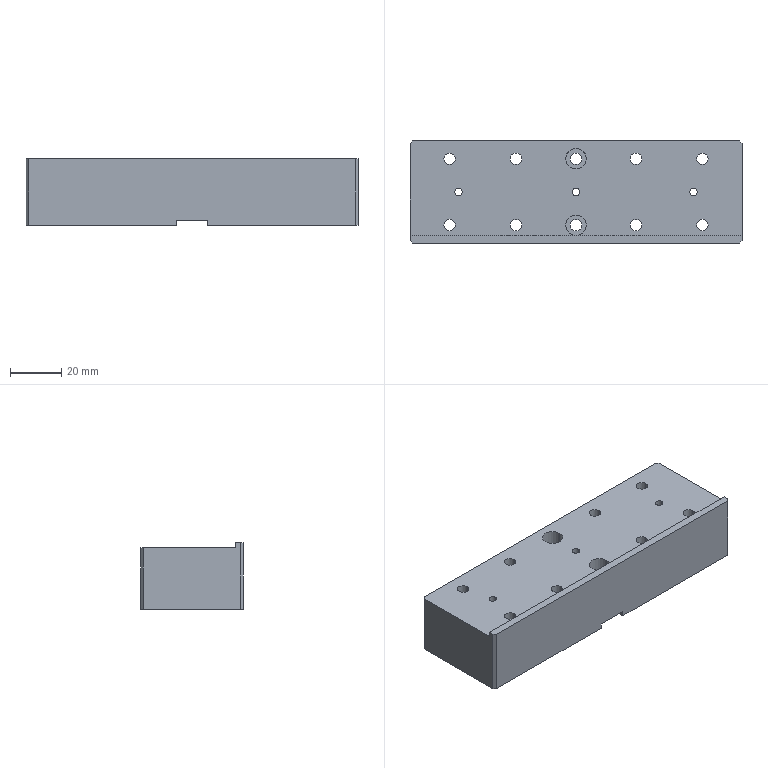Part | STEP file | 1 solid | 97 faces | box 130 x 40 x 26 mm | volume 113465 mm3 | cylinder 60 | plane 29 | cone 8 | commonest cylinder face diameters 4.5 x20 8 x20 4.2 x8 3 x6 4 x6